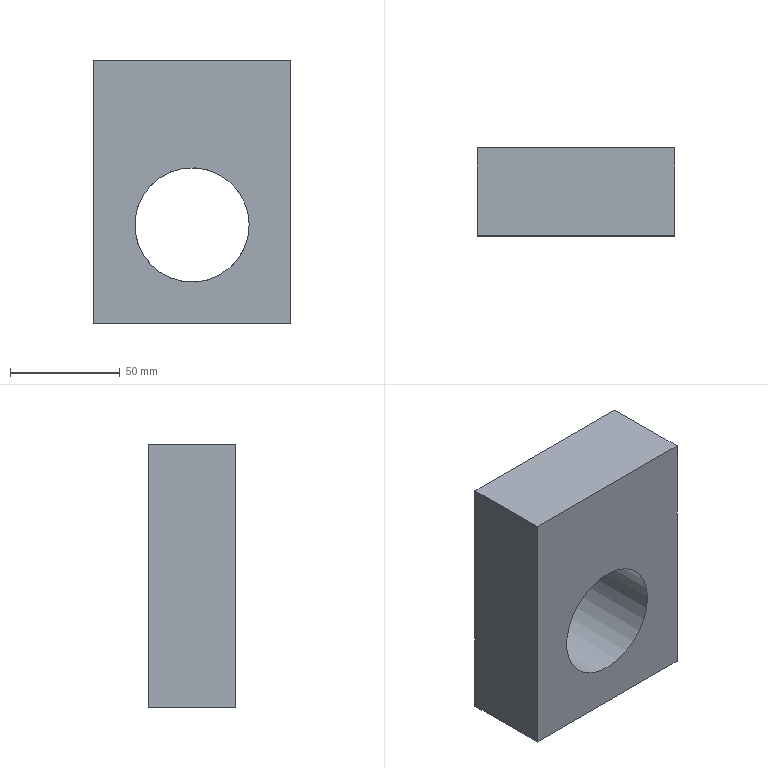Part | NX | features solid 2 | 1 solid | 7 faces | box 90 x 40 x 120 mm | volume 347051 mm3 | plane 6 | cylinder 1 | commonest cylinder face diameters 52 x1
STEP:
#1=CARTESIAN_POINT('',(-888.,245.324,155.));
#2=VERTEX_POINT('',#1);
#3=CARTESIAN_POINT('',(-798.,245.324,155.));
#4=VERTEX_POINT('',#3);
#5=CARTESIAN_POINT('',(-843.,245.324,155.));
#6=DIRECTION('',(1.,0.,0.));
#7=VECTOR('',#6,1000.);
#8=LINE('',#5,#7);
#9=EDGE_CURVE('',#2,#4,#8,.T.);
#10=ORIENTED_EDGE('',*,*,#9,.T.);
#11=CARTESIAN_POINT('',(-798.,285.324,155.));
#12=VERTEX_POINT('',#11);
#13=CARTESIAN_POINT('',(-798.,270.324,155.));
#14=DIRECTION('',(0.,1.,0.));
#15=VECTOR('',#14,1000.);
#16=LINE('',#13,#15);
#17=EDGE_CURVE('',#4,#12,#16,.T.);
#18=ORIENTED_EDGE('',*,*,#17,.T.);
#19=CARTESIAN_POINT('',(-888.,285.324,155.));
#20=VERTEX_POINT('',#19);
#21=CARTESIAN_POINT('',(-843.,285.324,155.));
#22=DIRECTION('',(-1.,0.,0.));
#23=VECTOR('',#22,1000.);
#24=LINE('',#21,#23);
#25=EDGE_CURVE('',#12,#20,#24,.T.);
#26=ORIENTED_EDGE('',*,*,#25,.T.);
#27=CARTESIAN_POINT('',(-888.,270.324,155.));
#28=DIRECTION('',(0.,-1.,0.));
#29=VECTOR('',#28,1000.);
#30=LINE('',#27,#29);
#31=EDGE_CURVE('',#20,#2,#30,.T.);
#32=ORIENTED_EDGE('',*,*,#31,.T.);
#33=EDGE_LOOP('',(#10,#18,#26,#32));
#34=FACE_BOUND('',#33,.T.);
#35=CARTESIAN_POINT('',(-843.,270.324,155.));
#36=DIRECTION('',(0.,0.,1.));
#37=DIRECTION('',(-1.,0.,0.));
#38=AXIS2_PLACEMENT_3D('',#35,#36,#37);
#39=PLANE('',#38);
#40=ADVANCED_FACE('',(#34),#39,.T.);
#41=CARTESIAN_POINT('',(-817.,245.324,80.));
#42=VERTEX_POINT('',#41);
#43=CARTESIAN_POINT('',(-843.,245.324,80.));
#44=DIRECTION('',(0.,-1.,0.));
#45=DIRECTION('',(1.,0.,0.));
#46=AXIS2_PLACEMENT_3D('',#43,#44,#45);
#47=CIRCLE('',#46,26.);
#48=EDGE_CURVE('',#42,#42,#47,.F.);
#49=ORIENTED_EDGE('',*,*,#48,.T.);
#50=EDGE_LOOP('',(#49));
#51=FACE_BOUND('',#50,.T.);
#52=CARTESIAN_POINT('',(-888.,245.324,35.));
#53=VERTEX_POINT('',#52);
#54=CARTESIAN_POINT('',(-888.,245.324,35.));
#55=DIRECTION('',(0.,0.,1.));
#56=VECTOR('',#55,1000.);
#57=LINE('',#54,#56);
#58=EDGE_CURVE('',#53,#2,#57,.T.);
#59=ORIENTED_EDGE('',*,*,#58,.F.);
#60=CARTESIAN_POINT('',(-798.,245.324,35.));
#61=VERTEX_POINT('',#60);
#62=CARTESIAN_POINT('',(-843.,245.324,35.));
#63=DIRECTION('',(-1.,0.,0.));
#64=VECTOR('',#63,1000.);
#65=LINE('',#62,#64);
#66=EDGE_CURVE('',#61,#53,#65,.T.);
#67=ORIENTED_EDGE('',*,*,#66,.F.);
#68=CARTESIAN_POINT('',(-798.,245.324,35.));
#69=DIRECTION('',(0.,0.,1.));
#70=VECTOR('',#69,1000.);
#71=LINE('',#68,#70);
#72=EDGE_CURVE('',#61,#4,#71,.T.);
#73=ORIENTED_EDGE('',*,*,#72,.T.);
#74=ORIENTED_EDGE('',*,*,#9,.F.);
#75=EDGE_LOOP('',(#59,#67,#73,#74));
#76=FACE_BOUND('',#75,.T.);
#77=CARTESIAN_POINT('',(-843.,245.324,35.));
#78=DIRECTION('',(0.,-1.,0.));
#79=DIRECTION('',(0.,0.,-1.));
#80=AXIS2_PLACEMENT_3D('',#77,#78,#79);
#81=PLANE('',#80);
#82=ADVANCED_FACE('',(#51,#76),#81,.T.);
#83=ORIENTED_EDGE('',*,*,#72,.F.);
#84=CARTESIAN_POINT('',(-798.,285.324,35.));
#85=VERTEX_POINT('',#84);
#86=CARTESIAN_POINT('',(-798.,270.324,35.));
#87=DIRECTION('',(0.,-1.,0.));
#88=VECTOR('',#87,1000.);
#89=LINE('',#86,#88);
#90=EDGE_CURVE('',#85,#61,#89,.T.);
#91=ORIENTED_EDGE('',*,*,#90,.F.);
#92=CARTESIAN_POINT('',(-798.,285.324,35.));
#93=DIRECTION('',(0.,0.,1.));
#94=VECTOR('',#93,1000.);
#95=LINE('',#92,#94);
#96=EDGE_CURVE('',#85,#12,#95,.T.);
#97=ORIENTED_EDGE('',*,*,#96,.T.);
#98=ORIENTED_EDGE('',*,*,#17,.F.);
#99=EDGE_LOOP('',(#83,#91,#97,#98));
#100=FACE_BOUND('',#99,.T.);
#101=CARTESIAN_POINT('',(-798.,270.324,35.));
#102=DIRECTION('',(1.,0.,0.));
#103=DIRECTION('',(0.,0.,1.));
#104=AXIS2_PLACEMENT_3D('',#101,#102,#103);
#105=PLANE('',#104);
#106=ADVANCED_FACE('',(#100),#105,.T.);
#107=CARTESIAN_POINT('',(-843.,285.324,106.));
#108=VERTEX_POINT('',#107);
#109=CARTESIAN_POINT('',(-843.,285.324,80.));
#110=DIRECTION('',(0.,-1.,0.));
#111=DIRECTION('',(0.,0.,1.));
#112=AXIS2_PLACEMENT_3D('',#109,#110,#111);
#113=CIRCLE('',#112,26.);
#114=EDGE_CURVE('',#108,#108,#113,.T.);
#115=ORIENTED_EDGE('',*,*,#114,.T.);
#116=EDGE_LOOP('',(#115));
#117=FACE_BOUND('',#116,.T.);
#118=ORIENTED_EDGE('',*,*,#96,.F.);
#119=CARTESIAN_POINT('',(-888.,285.324,35.));
#120=VERTEX_POINT('',#119);
#121=CARTESIAN_POINT('',(-843.,285.324,35.));
#122=DIRECTION('',(1.,0.,0.));
#123=VECTOR('',#122,1000.);
#124=LINE('',#121,#123);
#125=EDGE_CURVE('',#120,#85,#124,.T.);
#126=ORIENTED_EDGE('',*,*,#125,.F.);
#127=CARTESIAN_POINT('',(-888.,285.324,35.));
#128=DIRECTION('',(0.,0.,1.));
#129=VECTOR('',#128,1000.);
#130=LINE('',#127,#129);
#131=EDGE_CURVE('',#120,#20,#130,.T.);
#132=ORIENTED_EDGE('',*,*,#131,.T.);
#133=ORIENTED_EDGE('',*,*,#25,.F.);
#134=EDGE_LOOP('',(#118,#126,#132,#133));
#135=FACE_BOUND('',#134,.T.);
#136=CARTESIAN_POINT('',(-843.,285.324,35.));
#137=DIRECTION('',(0.,1.,0.));
#138=DIRECTION('',(0.,0.,1.));
#139=AXIS2_PLACEMENT_3D('',#136,#137,#138);
#140=PLANE('',#139);
#141=ADVANCED_FACE('',(#117,#135),#140,.T.);
#142=CARTESIAN_POINT('',(-888.,270.324,35.));
#143=DIRECTION('',(0.,1.,0.));
#144=VECTOR('',#143,1000.);
#145=LINE('',#142,#144);
#146=EDGE_CURVE('',#53,#120,#145,.T.);
#147=ORIENTED_EDGE('',*,*,#146,.T.);
#148=ORIENTED_EDGE('',*,*,#125,.T.);
#149=ORIENTED_EDGE('',*,*,#90,.T.);
#150=ORIENTED_EDGE('',*,*,#66,.T.);
#151=EDGE_LOOP('',(#147,#148,#149,#150));
#152=FACE_BOUND('',#151,.T.);
#153=CARTESIAN_POINT('',(-843.,270.324,35.));
#154=DIRECTION('',(0.,0.,-1.));
#155=DIRECTION('',(1.,0.,0.));
#156=AXIS2_PLACEMENT_3D('',#153,#154,#155);
#157=PLANE('',#156);
#158=ADVANCED_FACE('',(#152),#157,.T.);
#159=ORIENTED_EDGE('',*,*,#146,.F.);
#160=ORIENTED_EDGE('',*,*,#58,.T.);
#161=ORIENTED_EDGE('',*,*,#31,.F.);
#162=ORIENTED_EDGE('',*,*,#131,.F.);
#163=EDGE_LOOP('',(#159,#160,#161,#162));
#164=FACE_BOUND('',#163,.T.);
#165=CARTESIAN_POINT('',(-888.,270.324,35.));
#166=DIRECTION('',(-1.,0.,0.));
#167=DIRECTION('',(0.,0.,-1.));
#168=AXIS2_PLACEMENT_3D('',#165,#166,#167);
#169=PLANE('',#168);
#170=ADVANCED_FACE('',(#164),#169,.T.);
#171=ORIENTED_EDGE('',*,*,#48,.F.);
#172=EDGE_LOOP('',(#171));
#173=FACE_BOUND('',#172,.T.);
#174=ORIENTED_EDGE('',*,*,#114,.F.);
#175=EDGE_LOOP('',(#174));
#176=FACE_BOUND('',#175,.T.);
#177=CARTESIAN_POINT('',(-843.,331.324,80.));
#178=DIRECTION('',(0.,-1.,0.));
#179=DIRECTION('',(0.,0.,-1.));
#180=AXIS2_PLACEMENT_3D('',#177,#178,#179);
#181=CYLINDRICAL_SURFACE('',#180,26.);
#182=ADVANCED_FACE('',(#173,#176),#181,.F.);
#183=CLOSED_SHELL('',(#40,#82,#106,#141,#158,#170,#182));
#184=MANIFOLD_SOLID_BREP('',#183);
#185=(LENGTH_UNIT()NAMED_UNIT(*)SI_UNIT(.MILLI.,.METRE.));
#186=UNCERTAINTY_MEASURE_WITH_UNIT(LENGTH_MEASURE(0.00001),#185,'','');
#187=(NAMED_UNIT(*)PLANE_ANGLE_UNIT()SI_UNIT($,.RADIAN.));
#188=(NAMED_UNIT(*)SI_UNIT($,.STERADIAN.)SOLID_ANGLE_UNIT());
#189=(GEOMETRIC_REPRESENTATION_CONTEXT(3)GLOBAL_UNCERTAINTY_ASSIGNED_CONTEXT((#186))GLOBAL_UNIT_ASSIGNED_CONTEXT((#185,#187,#188))REPRESENTATION_CONTEXT('',''));
#190=ADVANCED_BREP_SHAPE_REPRESENTATION('',(#184),#189);